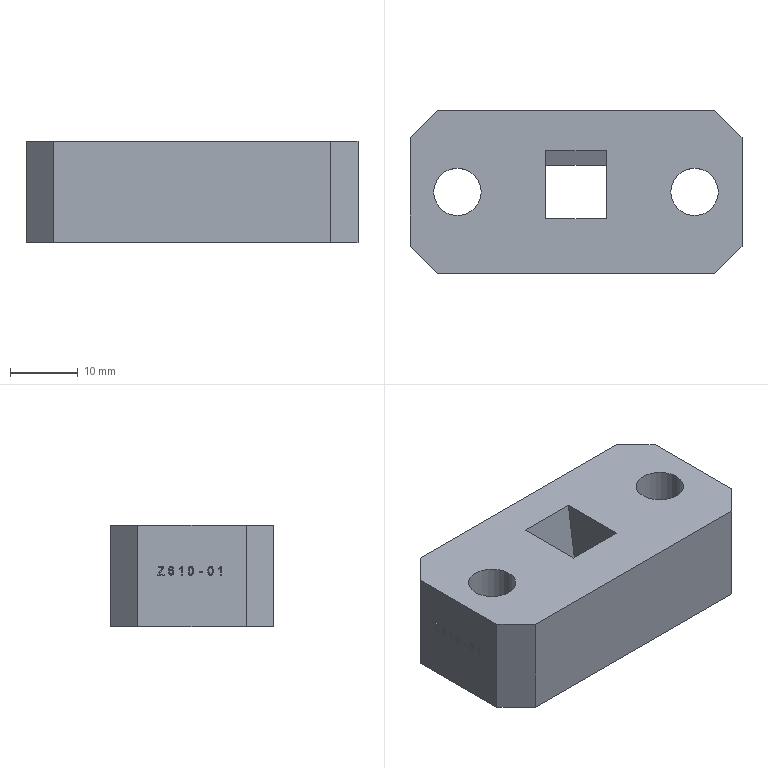Part | Creo | 1 solid | 136 faces | box 49 x 24 x 15 mm | volume 13850 mm3 | other 79 | plane 48 | cylinder 9 | commonest cylinder face diameters 7 x4 11 x4 17.925 x1